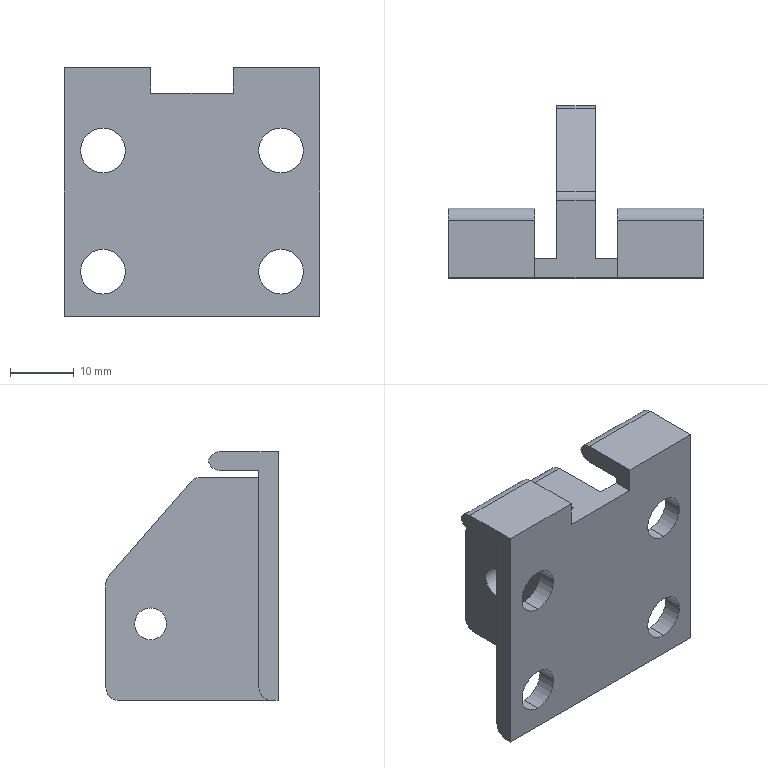Part | SolidWorks | features ICE 4, Extrusion 1, Fillet 1 | 1 solid | 36 faces | box 40 x 27 x 39 mm | volume 8879 mm3 | cylinder 19 | plane 17 | commonest cylinder face diameters 4 x9 7 x8 5 x2
STEP:
#1=CARTESIAN_POINT('',(13.951,3.,-16.5));
#2=VERTEX_POINT('',#1);
#3=CARTESIAN_POINT('',(13.951,3.,-9.5));
#4=VERTEX_POINT('',#3);
#5=CARTESIAN_POINT('',(13.951,3.,-13.));
#6=DIRECTION('',(0.,1.,0.));
#7=DIRECTION('',(0.,0.,-1.));
#8=AXIS2_PLACEMENT_3D('',#5,#6,#7);
#9=CIRCLE('',#8,3.5);
#10=EDGE_CURVE('',#2,#4,#9,.T.);
#11=ORIENTED_EDGE('',*,*,#10,.T.);
#12=CARTESIAN_POINT('',(13.951,0.,-9.5));
#13=VERTEX_POINT('',#12);
#14=CARTESIAN_POINT('',(13.951,27.001,-9.5));
#15=DIRECTION('',(0.,-1.,0.));
#16=VECTOR('',#15,1000.);
#17=LINE('',#14,#16);
#18=EDGE_CURVE('',#4,#13,#17,.T.);
#19=ORIENTED_EDGE('',*,*,#18,.T.);
#20=CARTESIAN_POINT('',(13.951,0.,-16.5));
#21=VERTEX_POINT('',#20);
#22=CARTESIAN_POINT('',(13.951,0.,-13.));
#23=DIRECTION('',(0.,-1.,0.));
#24=DIRECTION('',(0.,0.,1.));
#25=AXIS2_PLACEMENT_3D('',#22,#23,#24);
#26=CIRCLE('',#25,3.5);
#27=EDGE_CURVE('',#13,#21,#26,.T.);
#28=ORIENTED_EDGE('',*,*,#27,.T.);
#29=CARTESIAN_POINT('',(13.951,27.001,-16.5));
#30=DIRECTION('',(0.,-1.,0.));
#31=VECTOR('',#30,1000.);
#32=LINE('',#29,#31);
#33=EDGE_CURVE('',#2,#21,#32,.T.);
#34=ORIENTED_EDGE('',*,*,#33,.F.);
#35=EDGE_LOOP('',(#11,#19,#28,#34));
#36=FACE_OUTER_BOUND('',#35,.T.);
#37=CARTESIAN_POINT('',(13.951,27.001,-13.));
#38=DIRECTION('',(0.,-1.,0.));
#39=DIRECTION('',(0.,0.,-1.));
#40=AXIS2_PLACEMENT_3D('',#37,#38,#39);
#41=CYLINDRICAL_SURFACE('',#40,3.5);
#42=ADVANCED_FACE('',(#36),#41,.F.);
#43=CARTESIAN_POINT('',(13.951,3.,-35.5));
#44=VERTEX_POINT('',#43);
#45=CARTESIAN_POINT('',(13.951,3.,-28.5));
#46=VERTEX_POINT('',#45);
#47=CARTESIAN_POINT('',(13.951,3.,-32.));
#48=DIRECTION('',(0.,1.,0.));
#49=DIRECTION('',(0.,0.,-1.));
#50=AXIS2_PLACEMENT_3D('',#47,#48,#49);
#51=CIRCLE('',#50,3.5);
#52=EDGE_CURVE('',#44,#46,#51,.T.);
#53=ORIENTED_EDGE('',*,*,#52,.T.);
#54=CARTESIAN_POINT('',(13.951,0.,-28.5));
#55=VERTEX_POINT('',#54);
#56=CARTESIAN_POINT('',(13.951,27.001,-28.5));
#57=DIRECTION('',(0.,-1.,0.));
#58=VECTOR('',#57,1000.);
#59=LINE('',#56,#58);
#60=EDGE_CURVE('',#46,#55,#59,.T.);
#61=ORIENTED_EDGE('',*,*,#60,.T.);
#62=CARTESIAN_POINT('',(13.951,0.,-35.5));
#63=VERTEX_POINT('',#62);
#64=CARTESIAN_POINT('',(13.951,0.,-32.));
#65=DIRECTION('',(0.,-1.,0.));
#66=DIRECTION('',(0.,0.,1.));
#67=AXIS2_PLACEMENT_3D('',#64,#65,#66);
#68=CIRCLE('',#67,3.5);
#69=EDGE_CURVE('',#55,#63,#68,.T.);
#70=ORIENTED_EDGE('',*,*,#69,.T.);
#71=CARTESIAN_POINT('',(13.951,27.001,-35.5));
#72=DIRECTION('',(0.,-1.,0.));
#73=VECTOR('',#72,1000.);
#74=LINE('',#71,#73);
#75=EDGE_CURVE('',#44,#63,#74,.T.);
#76=ORIENTED_EDGE('',*,*,#75,.F.);
#77=EDGE_LOOP('',(#53,#61,#70,#76));
#78=FACE_OUTER_BOUND('',#77,.T.);
#79=CARTESIAN_POINT('',(13.951,27.001,-32.));
#80=DIRECTION('',(0.,-1.,0.));
#81=DIRECTION('',(0.,0.,-1.));
#82=AXIS2_PLACEMENT_3D('',#79,#80,#81);
#83=CYLINDRICAL_SURFACE('',#82,3.5);
#84=ADVANCED_FACE('',(#78),#83,.F.);
#85=CARTESIAN_POINT('',(-13.951,3.,-35.5));
#86=VERTEX_POINT('',#85);
#87=CARTESIAN_POINT('',(-13.951,3.,-28.5));
#88=VERTEX_POINT('',#87);
#89=CARTESIAN_POINT('',(-13.951,3.,-32.));
#90=DIRECTION('',(0.,1.,0.));
#91=DIRECTION('',(0.,0.,-1.));
#92=AXIS2_PLACEMENT_3D('',#89,#90,#91);
#93=CIRCLE('',#92,3.5);
#94=EDGE_CURVE('',#86,#88,#93,.T.);
#95=ORIENTED_EDGE('',*,*,#94,.T.);
#96=CARTESIAN_POINT('',(-13.951,0.,-28.5));
#97=VERTEX_POINT('',#96);
#98=CARTESIAN_POINT('',(-13.951,27.001,-28.5));
#99=DIRECTION('',(0.,-1.,0.));
#100=VECTOR('',#99,1000.);
#101=LINE('',#98,#100);
#102=EDGE_CURVE('',#88,#97,#101,.T.);
#103=ORIENTED_EDGE('',*,*,#102,.T.);
#104=CARTESIAN_POINT('',(-13.951,0.,-35.5));
#105=VERTEX_POINT('',#104);
#106=CARTESIAN_POINT('',(-13.951,0.,-32.));
#107=DIRECTION('',(0.,-1.,0.));
#108=DIRECTION('',(0.,0.,-1.));
#109=AXIS2_PLACEMENT_3D('',#106,#107,#108);
#110=CIRCLE('',#109,3.5);
#111=EDGE_CURVE('',#97,#105,#110,.T.);
#112=ORIENTED_EDGE('',*,*,#111,.T.);
#113=CARTESIAN_POINT('',(-13.951,27.001,-35.5));
#114=DIRECTION('',(0.,-1.,0.));
#115=VECTOR('',#114,1000.);
#116=LINE('',#113,#115);
#117=EDGE_CURVE('',#86,#105,#116,.T.);
#118=ORIENTED_EDGE('',*,*,#117,.F.);
#119=EDGE_LOOP('',(#95,#103,#112,#118));
#120=FACE_OUTER_BOUND('',#119,.T.);
#121=CARTESIAN_POINT('',(-13.951,27.001,-32.));
#122=DIRECTION('',(0.,-1.,0.));
#123=DIRECTION('',(0.,0.,-1.));
#124=AXIS2_PLACEMENT_3D('',#121,#122,#123);
#125=CYLINDRICAL_SURFACE('',#124,3.5);
#126=ADVANCED_FACE('',(#120),#125,.F.);
#127=CARTESIAN_POINT('',(-13.951,3.,-16.5));
#128=VERTEX_POINT('',#127);
#129=CARTESIAN_POINT('',(-13.951,3.,-9.5));
#130=VERTEX_POINT('',#129);
#131=CARTESIAN_POINT('',(-13.951,3.,-13.));
#132=DIRECTION('',(0.,1.,0.));
#133=DIRECTION('',(0.,0.,-1.));
#134=AXIS2_PLACEMENT_3D('',#131,#132,#133);
#135=CIRCLE('',#134,3.5);
#136=EDGE_CURVE('',#128,#130,#135,.T.);
#137=ORIENTED_EDGE('',*,*,#136,.T.);
#138=CARTESIAN_POINT('',(-13.951,0.,-9.5));
#139=VERTEX_POINT('',#138);
#140=CARTESIAN_POINT('',(-13.951,27.001,-9.5));
#141=DIRECTION('',(0.,-1.,0.));
#142=VECTOR('',#141,1000.);
#143=LINE('',#140,#142);
#144=EDGE_CURVE('',#130,#139,#143,.T.);
#145=ORIENTED_EDGE('',*,*,#144,.T.);
#146=CARTESIAN_POINT('',(-13.951,0.,-16.5));
#147=VERTEX_POINT('',#146);
#148=CARTESIAN_POINT('',(-13.951,0.,-13.));
#149=DIRECTION('',(0.,-1.,0.));
#150=DIRECTION('',(0.,0.,-1.));
#151=AXIS2_PLACEMENT_3D('',#148,#149,#150);
#152=CIRCLE('',#151,3.5);
#153=EDGE_CURVE('',#139,#147,#152,.T.);
#154=ORIENTED_EDGE('',*,*,#153,.T.);
#155=CARTESIAN_POINT('',(-13.951,27.001,-16.5));
#156=DIRECTION('',(0.,-1.,0.));
#157=VECTOR('',#156,1000.);
#158=LINE('',#155,#157);
#159=EDGE_CURVE('',#128,#147,#158,.T.);
#160=ORIENTED_EDGE('',*,*,#159,.F.);
#161=EDGE_LOOP('',(#137,#145,#154,#160));
#162=FACE_OUTER_BOUND('',#161,.T.);
#163=CARTESIAN_POINT('',(-13.951,27.001,-13.));
#164=DIRECTION('',(0.,-1.,0.));
#165=DIRECTION('',(0.,0.,-1.));
#166=AXIS2_PLACEMENT_3D('',#163,#164,#165);
#167=CYLINDRICAL_SURFACE('',#166,3.5);
#168=ADVANCED_FACE('',(#162),#167,.F.);
#169=CARTESIAN_POINT('',(-3.,20.,-29.5));
#170=VERTEX_POINT('',#169);
#171=CARTESIAN_POINT('',(-3.,20.,-24.5));
#172=VERTEX_POINT('',#171);
#173=CARTESIAN_POINT('',(-3.,20.,-27.));
#174=DIRECTION('',(-1.,0.,0.));
#175=DIRECTION('',(0.,0.,-1.));
#176=AXIS2_PLACEMENT_3D('',#173,#174,#175);
#177=CIRCLE('',#176,2.5);
#178=EDGE_CURVE('',#170,#172,#177,.T.);
#179=ORIENTED_EDGE('',*,*,#178,.T.);
#180=CARTESIAN_POINT('',(3.,20.,-24.5));
#181=VERTEX_POINT('',#180);
#182=CARTESIAN_POINT('',(-20.001,20.,-24.5));
#183=DIRECTION('',(1.,0.,0.));
#184=VECTOR('',#183,1000.);
#185=LINE('',#182,#184);
#186=EDGE_CURVE('',#172,#181,#185,.T.);
#187=ORIENTED_EDGE('',*,*,#186,.T.);
#188=CARTESIAN_POINT('',(3.,20.,-29.5));
#189=VERTEX_POINT('',#188);
#190=CARTESIAN_POINT('',(3.,20.,-27.));
#191=DIRECTION('',(1.,0.,0.));
#192=DIRECTION('',(0.,0.,-1.));
#193=AXIS2_PLACEMENT_3D('',#190,#191,#192);
#194=CIRCLE('',#193,2.5);
#195=EDGE_CURVE('',#181,#189,#194,.T.);
#196=ORIENTED_EDGE('',*,*,#195,.T.);
#197=CARTESIAN_POINT('',(-20.001,20.,-29.5));
#198=DIRECTION('',(1.,0.,0.));
#199=VECTOR('',#198,1000.);
#200=LINE('',#197,#199);
#201=EDGE_CURVE('',#170,#189,#200,.T.);
#202=ORIENTED_EDGE('',*,*,#201,.F.);
#203=EDGE_LOOP('',(#179,#187,#196,#202));
#204=FACE_OUTER_BOUND('',#203,.T.);
#205=CARTESIAN_POINT('',(-20.001,20.,-27.));
#206=DIRECTION('',(1.,0.,0.));
#207=DIRECTION('',(0.,0.,-1.));
#208=AXIS2_PLACEMENT_3D('',#205,#206,#207);
#209=CYLINDRICAL_SURFACE('',#208,2.5);
#210=ADVANCED_FACE('',(#204),#209,.F.);
#211=ORIENTED_EDGE('',*,*,#94,.F.);
#212=CARTESIAN_POINT('',(-13.951,3.,-32.));
#213=DIRECTION('',(0.,1.,0.));
#214=DIRECTION('',(0.,0.,-1.));
#215=AXIS2_PLACEMENT_3D('',#212,#213,#214);
#216=CIRCLE('',#215,3.5);
#217=EDGE_CURVE('',#88,#86,#216,.T.);
#218=ORIENTED_EDGE('',*,*,#217,.F.);
#219=EDGE_LOOP('',(#211,#218));
#220=FACE_BOUND('',#219,.T.);
#221=ORIENTED_EDGE('',*,*,#136,.F.);
#222=CARTESIAN_POINT('',(-13.951,3.,-13.));
#223=DIRECTION('',(0.,1.,0.));
#224=DIRECTION('',(0.,0.,-1.));
#225=AXIS2_PLACEMENT_3D('',#222,#223,#224);
#226=CIRCLE('',#225,3.5);
#227=EDGE_CURVE('',#130,#128,#226,.T.);
#228=ORIENTED_EDGE('',*,*,#227,.F.);
#229=EDGE_LOOP('',(#221,#228));
#230=FACE_BOUND('',#229,.T.);
#231=CARTESIAN_POINT('',(-3.,3.,-4.));
#232=VERTEX_POINT('',#231);
#233=CARTESIAN_POINT('',(-3.,3.,-37.));
#234=VERTEX_POINT('',#233);
#235=CARTESIAN_POINT('',(-3.,3.,-4.));
#236=DIRECTION('',(0.,0.,-1.));
#237=VECTOR('',#236,1000.);
#238=LINE('',#235,#237);
#239=EDGE_CURVE('',#232,#234,#238,.T.);
#240=ORIENTED_EDGE('',*,*,#239,.T.);
#241=CARTESIAN_POINT('',(-20.,3.,-37.));
#242=VERTEX_POINT('',#241);
#243=CARTESIAN_POINT('',(20.,3.,-37.));
#244=DIRECTION('',(-1.,0.,0.));
#245=VECTOR('',#244,1000.);
#246=LINE('',#243,#245);
#247=EDGE_CURVE('',#234,#242,#246,.T.);
#248=ORIENTED_EDGE('',*,*,#247,.T.);
#249=CARTESIAN_POINT('',(-20.,3.,-3.));
#250=VERTEX_POINT('',#249);
#251=CARTESIAN_POINT('',(-20.,3.,0.));
#252=DIRECTION('',(0.,0.,1.));
#253=VECTOR('',#252,1000.);
#254=LINE('',#251,#253);
#255=EDGE_CURVE('',#242,#250,#254,.T.);
#256=ORIENTED_EDGE('',*,*,#255,.T.);
#257=CARTESIAN_POINT('',(-6.5,3.,-3.));
#258=VERTEX_POINT('',#257);
#259=CARTESIAN_POINT('',(20.,3.,-3.));
#260=DIRECTION('',(-1.,0.,0.));
#261=VECTOR('',#260,1000.);
#262=LINE('',#259,#261);
#263=EDGE_CURVE('',#258,#250,#262,.T.);
#264=ORIENTED_EDGE('',*,*,#263,.F.);
#265=CARTESIAN_POINT('',(-6.5,3.,-4.));
#266=VERTEX_POINT('',#265);
#267=CARTESIAN_POINT('',(-6.5,3.,0.));
#268=DIRECTION('',(0.,0.,1.));
#269=VECTOR('',#268,1000.);
#270=LINE('',#267,#269);
#271=EDGE_CURVE('',#266,#258,#270,.T.);
#272=ORIENTED_EDGE('',*,*,#271,.F.);
#273=CARTESIAN_POINT('',(20.,3.,-4.));
#274=DIRECTION('',(1.,0.,0.));
#275=VECTOR('',#274,1000.);
#276=LINE('',#273,#275);
#277=EDGE_CURVE('',#266,#232,#276,.T.);
#278=ORIENTED_EDGE('',*,*,#277,.T.);
#279=EDGE_LOOP('',(#240,#248,#256,#264,#272,#278));
#280=FACE_OUTER_BOUND('',#279,.T.);
#281=CARTESIAN_POINT('',(20.,3.,0.));
#282=DIRECTION('',(0.,-1.,0.));
#283=DIRECTION('',(0.,0.,-1.));
#284=AXIS2_PLACEMENT_3D('',#281,#282,#283);
#285=PLANE('',#284);
#286=ADVANCED_FACE('',(#220,#230,#280),#285,.F.);
#287=CARTESIAN_POINT('',(-20.,9.,-3.));
#288=VERTEX_POINT('',#287);
#289=CARTESIAN_POINT('',(-20.,0.,-3.));
#290=DIRECTION('',(0.,-1.,0.));
#291=VECTOR('',#290,1000.);
#292=LINE('',#289,#291);
#293=EDGE_CURVE('',#288,#250,#292,.T.);
#294=ORIENTED_EDGE('',*,*,#293,.F.);
#295=CARTESIAN_POINT('',(-6.5,9.,-3.));
#296=VERTEX_POINT('',#295);
#297=CARTESIAN_POINT('',(20.,9.,-3.));
#298=DIRECTION('',(1.,0.,0.));
#299=VECTOR('',#298,1000.);
#300=LINE('',#297,#299);
#301=EDGE_CURVE('',#288,#296,#300,.T.);
#302=ORIENTED_EDGE('',*,*,#301,.T.);
#303=CARTESIAN_POINT('',(-6.5,0.,-3.));
#304=DIRECTION('',(0.,-1.,0.));
#305=VECTOR('',#304,1000.);
#306=LINE('',#303,#305);
#307=EDGE_CURVE('',#296,#258,#306,.T.);
#308=ORIENTED_EDGE('',*,*,#307,.T.);
#309=ORIENTED_EDGE('',*,*,#263,.T.);
#310=EDGE_LOOP('',(#294,#302,#308,#309));
#311=FACE_OUTER_BOUND('',#310,.T.);
#312=CARTESIAN_POINT('',(20.,0.,-3.));
#313=DIRECTION('',(0.,0.,-1.));
#314=DIRECTION('',(-1.,0.,0.));
#315=AXIS2_PLACEMENT_3D('',#312,#313,#314);
#316=PLANE('',#315);
#317=ADVANCED_FACE('',(#311),#316,.T.);
#318=CARTESIAN_POINT('',(-6.5,9.,0.));
#319=VERTEX_POINT('',#318);
#320=CARTESIAN_POINT('',(-6.5,0.,0.));
#321=VERTEX_POINT('',#320);
#322=CARTESIAN_POINT('',(-6.5,11.,0.));
#323=DIRECTION('',(0.,-1.,0.));
#324=VECTOR('',#323,1000.);
#325=LINE('',#322,#324);
#326=EDGE_CURVE('',#319,#321,#325,.T.);
#327=ORIENTED_EDGE('',*,*,#326,.F.);
#328=CARTESIAN_POINT('',(-20.,9.,0.));
#329=VERTEX_POINT('',#328);
#330=CARTESIAN_POINT('',(20.,9.,0.));
#331=DIRECTION('',(-1.,0.,0.));
#332=VECTOR('',#331,1000.);
#333=LINE('',#330,#332);
#334=EDGE_CURVE('',#319,#329,#333,.T.);
#335=ORIENTED_EDGE('',*,*,#334,.T.);
#336=CARTESIAN_POINT('',(-20.,0.,0.));
#337=VERTEX_POINT('',#336);
#338=CARTESIAN_POINT('',(-20.,0.,0.));
#339=DIRECTION('',(0.,1.,0.));
#340=VECTOR('',#339,1000.);
#341=LINE('',#338,#340);
#342=EDGE_CURVE('',#337,#329,#341,.T.);
#343=ORIENTED_EDGE('',*,*,#342,.F.);
#344=CARTESIAN_POINT('',(20.,0.,0.));
#345=DIRECTION('',(-1.,0.,0.));
#346=VECTOR('',#345,1000.);
#347=LINE('',#344,#346);
#348=EDGE_CURVE('',#321,#337,#347,.T.);
#349=ORIENTED_EDGE('',*,*,#348,.F.);
#350=EDGE_LOOP('',(#327,#335,#343,#349));
#351=FACE_OUTER_BOUND('',#350,.T.);
#352=CARTESIAN_POINT('',(20.,0.,0.));
#353=DIRECTION('',(0.,0.,1.));
#354=DIRECTION('',(1.,0.,0.));
#355=AXIS2_PLACEMENT_3D('',#352,#353,#354);
#356=PLANE('',#355);
#357=ADVANCED_FACE('',(#351),#356,.T.);
#358=CARTESIAN_POINT('',(13.951,0.,-13.));
#359=DIRECTION('',(0.,-1.,0.));
#360=DIRECTION('',(0.,0.,1.));
#361=AXIS2_PLACEMENT_3D('',#358,#359,#360);
#362=CIRCLE('',#361,3.5);
#363=EDGE_CURVE('',#21,#13,#362,.T.);
#364=ORIENTED_EDGE('',*,*,#363,.F.);
#365=ORIENTED_EDGE('',*,*,#27,.F.);
#366=EDGE_LOOP('',(#364,#365));
#367=FACE_BOUND('',#366,.T.);
#368=CARTESIAN_POINT('',(13.951,0.,-32.));
#369=DIRECTION('',(0.,-1.,0.));
#370=DIRECTION('',(0.,0.,1.));
#371=AXIS2_PLACEMENT_3D('',#368,#369,#370);
#372=CIRCLE('',#371,3.5);
#373=EDGE_CURVE('',#63,#55,#372,.T.);
#374=ORIENTED_EDGE('',*,*,#373,.F.);
#375=ORIENTED_EDGE('',*,*,#69,.F.);
#376=EDGE_LOOP('',(#374,#375));
#377=FACE_BOUND('',#376,.T.);
#378=CARTESIAN_POINT('',(-13.951,0.,-32.));
#379=DIRECTION('',(0.,-1.,0.));
#380=DIRECTION('',(0.,0.,-1.));
#381=AXIS2_PLACEMENT_3D('',#378,#379,#380);
#382=CIRCLE('',#381,3.5);
#383=EDGE_CURVE('',#105,#97,#382,.T.);
#384=ORIENTED_EDGE('',*,*,#383,.F.);
#385=ORIENTED_EDGE('',*,*,#111,.F.);
#386=EDGE_LOOP('',(#384,#385));
#387=FACE_BOUND('',#386,.T.);
#388=CARTESIAN_POINT('',(-13.951,0.,-13.));
#389=DIRECTION('',(0.,-1.,0.));
#390=DIRECTION('',(0.,0.,-1.));
#391=AXIS2_PLACEMENT_3D('',#388,#389,#390);
#392=CIRCLE('',#391,3.5);
#393=EDGE_CURVE('',#147,#139,#392,.T.);
#394=ORIENTED_EDGE('',*,*,#393,.F.);
#395=ORIENTED_EDGE('',*,*,#153,.F.);
#396=EDGE_LOOP('',(#394,#395));
#397=FACE_BOUND('',#396,.T.);
#398=CARTESIAN_POINT('',(-6.5,0.,-4.));
#399=VERTEX_POINT('',#398);
#400=CARTESIAN_POINT('',(-6.5,0.,0.));
#401=DIRECTION('',(0.,0.,-1.));
#402=VECTOR('',#401,1000.);
#403=LINE('',#400,#402);
#404=EDGE_CURVE('',#321,#399,#403,.T.);
#405=ORIENTED_EDGE('',*,*,#404,.F.);
#406=ORIENTED_EDGE('',*,*,#348,.T.);
#407=CARTESIAN_POINT('',(-20.,0.,-39.));
#408=VERTEX_POINT('',#407);
#409=CARTESIAN_POINT('',(-20.,0.,0.));
#410=DIRECTION('',(0.,0.,-1.));
#411=VECTOR('',#410,1000.);
#412=LINE('',#409,#411);
#413=EDGE_CURVE('',#337,#408,#412,.T.);
#414=ORIENTED_EDGE('',*,*,#413,.T.);
#415=CARTESIAN_POINT('',(20.,0.,-39.));
#416=VERTEX_POINT('',#415);
#417=CARTESIAN_POINT('',(20.,0.,-39.));
#418=DIRECTION('',(-1.,0.,0.));
#419=VECTOR('',#418,1000.);
#420=LINE('',#417,#419);
#421=EDGE_CURVE('',#416,#408,#420,.T.);
#422=ORIENTED_EDGE('',*,*,#421,.F.);
#423=CARTESIAN_POINT('',(20.,0.,0.));
#424=VERTEX_POINT('',#423);
#425=CARTESIAN_POINT('',(20.,0.,0.));
#426=DIRECTION('',(0.,0.,-1.));
#427=VECTOR('',#426,1000.);
#428=LINE('',#425,#427);
#429=EDGE_CURVE('',#424,#416,#428,.T.);
#430=ORIENTED_EDGE('',*,*,#429,.F.);
#431=CARTESIAN_POINT('',(6.5,0.,0.));
#432=VERTEX_POINT('',#431);
#433=CARTESIAN_POINT('',(20.,0.,0.));
#434=DIRECTION('',(-1.,0.,0.));
#435=VECTOR('',#434,1000.);
#436=LINE('',#433,#435);
#437=EDGE_CURVE('',#424,#432,#436,.T.);
#438=ORIENTED_EDGE('',*,*,#437,.T.);
#439=CARTESIAN_POINT('',(6.5,0.,-4.));
#440=VERTEX_POINT('',#439);
#441=CARTESIAN_POINT('',(6.5,0.,0.));
#442=DIRECTION('',(0.,0.,-1.));
#443=VECTOR('',#442,1000.);
#444=LINE('',#441,#443);
#445=EDGE_CURVE('',#432,#440,#444,.T.);
#446=ORIENTED_EDGE('',*,*,#445,.T.);
#447=CARTESIAN_POINT('',(-6.5,0.,-4.));
#448=DIRECTION('',(1.,0.,0.));
#449=VECTOR('',#448,1000.);
#450=LINE('',#447,#449);
#451=EDGE_CURVE('',#399,#440,#450,.T.);
#452=ORIENTED_EDGE('',*,*,#451,.F.);
#453=EDGE_LOOP('',(#405,#406,#414,#422,#430,#438,#446,#452));
#454=FACE_OUTER_BOUND('',#453,.T.);
#455=CARTESIAN_POINT('',(20.,0.,0.));
#456=DIRECTION('',(0.,1.,0.));
#457=DIRECTION('',(0.,0.,1.));
#458=AXIS2_PLACEMENT_3D('',#455,#456,#457);
#459=PLANE('',#458);
#460=ADVANCED_FACE('',(#367,#377,#387,#397,#454),#459,.F.);
#461=ORIENTED_EDGE('',*,*,#10,.F.);
#462=CARTESIAN_POINT('',(13.951,3.,-13.));
#463=DIRECTION('',(0.,1.,0.));
#464=DIRECTION('',(0.,0.,-1.));
#465=AXIS2_PLACEMENT_3D('',#462,#463,#464);
#466=CIRCLE('',#465,3.5);
#467=EDGE_CURVE('',#4,#2,#466,.T.);
#468=ORIENTED_EDGE('',*,*,#467,.F.);
#469=EDGE_LOOP('',(#461,#468));
#470=FACE_BOUND('',#469,.T.);
#471=ORIENTED_EDGE('',*,*,#52,.F.);
#472=CARTESIAN_POINT('',(13.951,3.,-32.));
#473=DIRECTION('',(0.,1.,0.));
#474=DIRECTION('',(0.,0.,-1.));
#475=AXIS2_PLACEMENT_3D('',#472,#473,#474);
#476=CIRCLE('',#475,3.5);
#477=EDGE_CURVE('',#46,#44,#476,.T.);
#478=ORIENTED_EDGE('',*,*,#477,.F.);
#479=EDGE_LOOP('',(#471,#478));
#480=FACE_BOUND('',#479,.T.);
#481=CARTESIAN_POINT('',(20.,3.,-37.));
#482=VERTEX_POINT('',#481);
#483=CARTESIAN_POINT('',(20.,3.,-3.));
#484=VERTEX_POINT('',#483);
#485=CARTESIAN_POINT('',(20.,3.,0.));
#486=DIRECTION('',(0.,0.,1.));
#487=VECTOR('',#486,1000.);
#488=LINE('',#485,#487);
#489=EDGE_CURVE('',#482,#484,#488,.T.);
#490=ORIENTED_EDGE('',*,*,#489,.F.);
#491=CARTESIAN_POINT('',(3.,3.,-37.));
#492=VERTEX_POINT('',#491);
#493=CARTESIAN_POINT('',(20.,3.,-37.));
#494=DIRECTION('',(-1.,0.,0.));
#495=VECTOR('',#494,1000.);
#496=LINE('',#493,#495);
#497=EDGE_CURVE('',#482,#492,#496,.T.);
#498=ORIENTED_EDGE('',*,*,#497,.T.);
#499=CARTESIAN_POINT('',(3.,3.,-4.));
#500=VERTEX_POINT('',#499);
#501=CARTESIAN_POINT('',(3.,3.,-4.));
#502=DIRECTION('',(0.,0.,-1.));
#503=VECTOR('',#502,1000.);
#504=LINE('',#501,#503);
#505=EDGE_CURVE('',#500,#492,#504,.T.);
#506=ORIENTED_EDGE('',*,*,#505,.F.);
#507=CARTESIAN_POINT('',(6.5,3.,-4.));
#508=VERTEX_POINT('',#507);
#509=CARTESIAN_POINT('',(20.,3.,-4.));
#510=DIRECTION('',(1.,0.,0.));
#511=VECTOR('',#510,1000.);
#512=LINE('',#509,#511);
#513=EDGE_CURVE('',#500,#508,#512,.T.);
#514=ORIENTED_EDGE('',*,*,#513,.T.);
#515=CARTESIAN_POINT('',(6.5,3.,-3.));
#516=VERTEX_POINT('',#515);
#517=CARTESIAN_POINT('',(6.5,3.,0.));
#518=DIRECTION('',(0.,0.,1.));
#519=VECTOR('',#518,1000.);
#520=LINE('',#517,#519);
#521=EDGE_CURVE('',#508,#516,#520,.T.);
#522=ORIENTED_EDGE('',*,*,#521,.T.);
#523=CARTESIAN_POINT('',(20.,3.,-3.));
#524=DIRECTION('',(-1.,0.,0.));
#525=VECTOR('',#524,1000.);
#526=LINE('',#523,#525);
#527=EDGE_CURVE('',#484,#516,#526,.T.);
#528=ORIENTED_EDGE('',*,*,#527,.F.);
#529=EDGE_LOOP('',(#490,#498,#506,#514,#522,#528));
#530=FACE_OUTER_BOUND('',#529,.T.);
#531=CARTESIAN_POINT('',(20.,3.,0.));
#532=DIRECTION('',(0.,-1.,0.));
#533=DIRECTION('',(0.,0.,-1.));
#534=AXIS2_PLACEMENT_3D('',#531,#532,#533);
#535=PLANE('',#534);
#536=ADVANCED_FACE('',(#470,#480,#530),#535,.F.);
#537=CARTESIAN_POINT('',(6.5,9.,-3.));
#538=VERTEX_POINT('',#537);
#539=CARTESIAN_POINT('',(6.5,0.,-3.));
#540=DIRECTION('',(0.,-1.,0.));
#541=VECTOR('',#540,1000.);
#542=LINE('',#539,#541);
#543=EDGE_CURVE('',#538,#516,#542,.T.);
#544=ORIENTED_EDGE('',*,*,#543,.F.);
#545=CARTESIAN_POINT('',(20.,9.,-3.));
#546=VERTEX_POINT('',#545);
#547=CARTESIAN_POINT('',(20.,9.,-3.));
#548=DIRECTION('',(1.,0.,0.));
#549=VECTOR('',#548,1000.);
#550=LINE('',#547,#549);
#551=EDGE_CURVE('',#538,#546,#550,.T.);
#552=ORIENTED_EDGE('',*,*,#551,.T.);
#553=CARTESIAN_POINT('',(20.,0.,-3.));
#554=DIRECTION('',(0.,-1.,0.));
#555=VECTOR('',#554,1000.);
#556=LINE('',#553,#555);
#557=EDGE_CURVE('',#546,#484,#556,.T.);
#558=ORIENTED_EDGE('',*,*,#557,.T.);
#559=ORIENTED_EDGE('',*,*,#527,.T.);
#560=EDGE_LOOP('',(#544,#552,#558,#559));
#561=FACE_OUTER_BOUND('',#560,.T.);
#562=CARTESIAN_POINT('',(20.,0.,-3.));
#563=DIRECTION('',(0.,0.,-1.));
#564=DIRECTION('',(-1.,0.,0.));
#565=AXIS2_PLACEMENT_3D('',#562,#563,#564);
#566=PLANE('',#565);
#567=ADVANCED_FACE('',(#561),#566,.T.);
#568=CARTESIAN_POINT('',(20.,9.,0.));
#569=VERTEX_POINT('',#568);
#570=CARTESIAN_POINT('',(20.,0.,0.));
#571=DIRECTION('',(0.,1.,0.));
#572=VECTOR('',#571,1000.);
#573=LINE('',#570,#572);
#574=EDGE_CURVE('',#424,#569,#573,.T.);
#575=ORIENTED_EDGE('',*,*,#574,.T.);
#576=CARTESIAN_POINT('',(6.5,9.,0.));
#577=VERTEX_POINT('',#576);
#578=CARTESIAN_POINT('',(20.,9.,0.));
#579=DIRECTION('',(-1.,0.,0.));
#580=VECTOR('',#579,1000.);
#581=LINE('',#578,#580);
#582=EDGE_CURVE('',#569,#577,#581,.T.);
#583=ORIENTED_EDGE('',*,*,#582,.T.);
#584=CARTESIAN_POINT('',(6.5,11.,0.));
#585=DIRECTION('',(0.,-1.,0.));
#586=VECTOR('',#585,1000.);
#587=LINE('',#584,#586);
#588=EDGE_CURVE('',#577,#432,#587,.T.);
#589=ORIENTED_EDGE('',*,*,#588,.T.);
#590=ORIENTED_EDGE('',*,*,#437,.F.);
#591=EDGE_LOOP('',(#575,#583,#589,#590));
#592=FACE_OUTER_BOUND('',#591,.T.);
#593=CARTESIAN_POINT('',(20.,0.,0.));
#594=DIRECTION('',(0.,0.,1.));
#595=DIRECTION('',(1.,0.,0.));
#596=AXIS2_PLACEMENT_3D('',#593,#594,#595);
#597=PLANE('',#596);
#598=ADVANCED_FACE('',(#592),#597,.T.);
#599=CARTESIAN_POINT('',(-20.,1.,-39.));
#600=VERTEX_POINT('',#599);
#601=CARTESIAN_POINT('',(-20.,0.,-39.));
#602=DIRECTION('',(0.,1.,0.));
#603=VECTOR('',#602,1000.);
#604=LINE('',#601,#603);
#605=EDGE_CURVE('',#408,#600,#604,.T.);
#606=ORIENTED_EDGE('',*,*,#605,.T.);
#607=CARTESIAN_POINT('',(-3.,1.,-39.));
#608=VERTEX_POINT('',#607);
#609=CARTESIAN_POINT('',(20.,1.,-39.));
#610=DIRECTION('',(1.,0.,0.));
#611=VECTOR('',#610,1000.);
#612=LINE('',#609,#611);
#613=EDGE_CURVE('',#600,#608,#612,.T.);
#614=ORIENTED_EDGE('',*,*,#613,.T.);
#615=CARTESIAN_POINT('',(-3.,25.,-39.));
#616=VERTEX_POINT('',#615);
#617=CARTESIAN_POINT('',(-3.,3.,-39.));
#618=DIRECTION('',(0.,1.,0.));
#619=VECTOR('',#618,1000.);
#620=LINE('',#617,#619);
#621=EDGE_CURVE('',#608,#616,#620,.T.);
#622=ORIENTED_EDGE('',*,*,#621,.T.);
#623=CARTESIAN_POINT('',(3.,25.,-39.));
#624=VERTEX_POINT('',#623);
#625=CARTESIAN_POINT('',(20.,25.,-39.));
#626=DIRECTION('',(1.,0.,0.));
#627=VECTOR('',#626,1000.);
#628=LINE('',#625,#627);
#629=EDGE_CURVE('',#616,#624,#628,.T.);
#630=ORIENTED_EDGE('',*,*,#629,.T.);
#631=CARTESIAN_POINT('',(3.,1.,-39.));
#632=VERTEX_POINT('',#631);
#633=CARTESIAN_POINT('',(3.,3.,-39.));
#634=DIRECTION('',(0.,1.,0.));
#635=VECTOR('',#634,1000.);
#636=LINE('',#633,#635);
#637=EDGE_CURVE('',#632,#624,#636,.T.);
#638=ORIENTED_EDGE('',*,*,#637,.F.);
#639=CARTESIAN_POINT('',(20.,1.,-39.));
#640=VERTEX_POINT('',#639);
#641=CARTESIAN_POINT('',(20.,1.,-39.));
#642=DIRECTION('',(1.,0.,0.));
#643=VECTOR('',#642,1000.);
#644=LINE('',#641,#643);
#645=EDGE_CURVE('',#632,#640,#644,.T.);
#646=ORIENTED_EDGE('',*,*,#645,.T.);
#647=CARTESIAN_POINT('',(20.,0.,-39.));
#648=DIRECTION('',(0.,1.,0.));
#649=VECTOR('',#648,1000.);
#650=LINE('',#647,#649);
#651=EDGE_CURVE('',#416,#640,#650,.T.);
#652=ORIENTED_EDGE('',*,*,#651,.F.);
#653=ORIENTED_EDGE('',*,*,#421,.T.);
#654=EDGE_LOOP('',(#606,#614,#622,#630,#638,#646,#652,#653));
#655=FACE_OUTER_BOUND('',#654,.T.);
#656=CARTESIAN_POINT('',(20.,0.,-39.));
#657=DIRECTION('',(0.,0.,1.));
#658=DIRECTION('',(1.,0.,0.));
#659=AXIS2_PLACEMENT_3D('',#656,#657,#658);
#660=PLANE('',#659);
#661=ADVANCED_FACE('',(#655),#660,.F.);
#662=ORIENTED_EDGE('',*,*,#651,.T.);
#663=CARTESIAN_POINT('',(20.,1.,-37.));
#664=DIRECTION('',(1.,0.,0.));
#665=DIRECTION('',(0.,0.,-1.));
#666=AXIS2_PLACEMENT_3D('',#663,#664,#665);
#667=CIRCLE('',#666,2.);
#668=EDGE_CURVE('',#640,#482,#667,.T.);
#669=ORIENTED_EDGE('',*,*,#668,.T.);
#670=ORIENTED_EDGE('',*,*,#489,.T.);
#671=ORIENTED_EDGE('',*,*,#557,.F.);
#672=CARTESIAN_POINT('',(20.,10.936,-1.5));
#673=VERTEX_POINT('',#672);
#674=CARTESIAN_POINT('',(20.,9.,-1.));
#675=DIRECTION('',(1.,0.,0.));
#676=DIRECTION('',(0.,0.,-1.));
#677=AXIS2_PLACEMENT_3D('',#674,#675,#676);
#678=CIRCLE('',#677,2.);
#679=EDGE_CURVE('',#546,#673,#678,.T.);
#680=ORIENTED_EDGE('',*,*,#679,.T.);
#681=CARTESIAN_POINT('',(20.,9.,-2.));
#682=DIRECTION('',(1.,0.,0.));
#683=DIRECTION('',(0.,0.,-1.));
#684=AXIS2_PLACEMENT_3D('',#681,#682,#683);
#685=CIRCLE('',#684,2.);
#686=EDGE_CURVE('',#673,#569,#685,.T.);
#687=ORIENTED_EDGE('',*,*,#686,.T.);
#688=ORIENTED_EDGE('',*,*,#574,.F.);
#689=ORIENTED_EDGE('',*,*,#429,.T.);
#690=EDGE_LOOP('',(#662,#669,#670,#671,#680,#687,#688,#689));
#691=FACE_OUTER_BOUND('',#690,.T.);
#692=CARTESIAN_POINT('',(20.,0.,0.));
#693=DIRECTION('',(1.,0.,0.));
#694=DIRECTION('',(0.,0.,-1.));
#695=AXIS2_PLACEMENT_3D('',#692,#693,#694);
#696=PLANE('',#695);
#697=ADVANCED_FACE('',(#691),#696,.T.);
#698=ORIENTED_EDGE('',*,*,#255,.F.);
#699=CARTESIAN_POINT('',(-20.,1.,-37.));
#700=DIRECTION('',(-1.,0.,0.));
#701=DIRECTION('',(0.,0.,-1.));
#702=AXIS2_PLACEMENT_3D('',#699,#700,#701);
#703=CIRCLE('',#702,2.);
#704=EDGE_CURVE('',#242,#600,#703,.T.);
#705=ORIENTED_EDGE('',*,*,#704,.T.);
#706=ORIENTED_EDGE('',*,*,#605,.F.);
#707=ORIENTED_EDGE('',*,*,#413,.F.);
#708=ORIENTED_EDGE('',*,*,#342,.T.);
#709=CARTESIAN_POINT('',(-20.,10.936,-1.5));
#710=VERTEX_POINT('',#709);
#711=CARTESIAN_POINT('',(-20.,9.,-2.));
#712=DIRECTION('',(-1.,0.,0.));
#713=DIRECTION('',(0.,0.,-1.));
#714=AXIS2_PLACEMENT_3D('',#711,#712,#713);
#715=CIRCLE('',#714,2.);
#716=EDGE_CURVE('',#329,#710,#715,.T.);
#717=ORIENTED_EDGE('',*,*,#716,.T.);
#718=CARTESIAN_POINT('',(-20.,9.,-1.));
#719=DIRECTION('',(-1.,0.,0.));
#720=DIRECTION('',(0.,0.,-1.));
#721=AXIS2_PLACEMENT_3D('',#718,#719,#720);
#722=CIRCLE('',#721,2.);
#723=EDGE_CURVE('',#710,#288,#722,.T.);
#724=ORIENTED_EDGE('',*,*,#723,.T.);
#725=ORIENTED_EDGE('',*,*,#293,.T.);
#726=EDGE_LOOP('',(#698,#705,#706,#707,#708,#717,#724,#725));
#727=FACE_OUTER_BOUND('',#726,.T.);
#728=CARTESIAN_POINT('',(-20.,0.,0.));
#729=DIRECTION('',(1.,0.,0.));
#730=DIRECTION('',(0.,0.,-1.));
#731=AXIS2_PLACEMENT_3D('',#728,#729,#730);
#732=PLANE('',#731);
#733=ADVANCED_FACE('',(#727),#732,.F.);
#734=CARTESIAN_POINT('',(3.,12.092,-4.));
#735=VERTEX_POINT('',#734);
#736=CARTESIAN_POINT('',(3.,13.,-4.));
#737=DIRECTION('',(0.,-1.,0.));
#738=VECTOR('',#737,1000.);
#739=LINE('',#736,#738);
#740=EDGE_CURVE('',#735,#500,#739,.T.);
#741=ORIENTED_EDGE('',*,*,#740,.F.);
#742=CARTESIAN_POINT('',(-3.,12.092,-4.));
#743=VERTEX_POINT('',#742);
#744=CARTESIAN_POINT('',(-6.5,12.092,-4.));
#745=DIRECTION('',(-1.,0.,0.));
#746=VECTOR('',#745,1000.);
#747=LINE('',#744,#746);
#748=EDGE_CURVE('',#735,#743,#747,.T.);
#749=ORIENTED_EDGE('',*,*,#748,.T.);
#750=CARTESIAN_POINT('',(-3.,13.,-4.));
#751=DIRECTION('',(0.,-1.,0.));
#752=VECTOR('',#751,1000.);
#753=LINE('',#750,#752);
#754=EDGE_CURVE('',#743,#232,#753,.T.);
#755=ORIENTED_EDGE('',*,*,#754,.T.);
#756=ORIENTED_EDGE('',*,*,#277,.F.);
#757=CARTESIAN_POINT('',(-6.5,11.,-4.));
#758=DIRECTION('',(0.,1.,0.));
#759=VECTOR('',#758,1000.);
#760=LINE('',#757,#759);
#761=EDGE_CURVE('',#399,#266,#760,.T.);
#762=ORIENTED_EDGE('',*,*,#761,.F.);
#763=ORIENTED_EDGE('',*,*,#451,.T.);
#764=CARTESIAN_POINT('',(6.5,11.,-4.));
#765=DIRECTION('',(0.,1.,0.));
#766=VECTOR('',#765,1000.);
#767=LINE('',#764,#766);
#768=EDGE_CURVE('',#440,#508,#767,.T.);
#769=ORIENTED_EDGE('',*,*,#768,.T.);
#770=ORIENTED_EDGE('',*,*,#513,.F.);
#771=EDGE_LOOP('',(#741,#749,#755,#756,#762,#763,#769,#770));
#772=FACE_OUTER_BOUND('',#771,.T.);
#773=CARTESIAN_POINT('',(-6.5,11.,-4.));
#774=DIRECTION('',(0.,0.,-1.));
#775=DIRECTION('',(0.,1.,0.));
#776=AXIS2_PLACEMENT_3D('',#773,#774,#775);
#777=PLANE('',#776);
#778=ADVANCED_FACE('',(#772),#777,.F.);
#779=ORIENTED_EDGE('',*,*,#307,.F.);
#780=CARTESIAN_POINT('',(-6.5,10.936,-1.5));
#781=VERTEX_POINT('',#780);
#782=CARTESIAN_POINT('',(-6.5,9.,-1.));
#783=DIRECTION('',(1.,0.,0.));
#784=DIRECTION('',(0.,0.,-1.));
#785=AXIS2_PLACEMENT_3D('',#782,#783,#784);
#786=CIRCLE('',#785,2.);
#787=EDGE_CURVE('',#296,#781,#786,.T.);
#788=ORIENTED_EDGE('',*,*,#787,.T.);
#789=CARTESIAN_POINT('',(-6.5,9.,-2.));
#790=DIRECTION('',(1.,0.,0.));
#791=DIRECTION('',(0.,0.,-1.));
#792=AXIS2_PLACEMENT_3D('',#789,#790,#791);
#793=CIRCLE('',#792,2.);
#794=EDGE_CURVE('',#781,#319,#793,.T.);
#795=ORIENTED_EDGE('',*,*,#794,.T.);
#796=ORIENTED_EDGE('',*,*,#326,.T.);
#797=ORIENTED_EDGE('',*,*,#404,.T.);
#798=ORIENTED_EDGE('',*,*,#761,.T.);
#799=ORIENTED_EDGE('',*,*,#271,.T.);
#800=EDGE_LOOP('',(#779,#788,#795,#796,#797,#798,#799));
#801=FACE_OUTER_BOUND('',#800,.T.);
#802=CARTESIAN_POINT('',(-6.5,0.,0.));
#803=DIRECTION('',(1.,0.,0.));
#804=DIRECTION('',(0.,0.,-1.));
#805=AXIS2_PLACEMENT_3D('',#802,#803,#804);
#806=PLANE('',#805);
#807=ADVANCED_FACE('',(#801),#806,.T.);
#808=CARTESIAN_POINT('',(6.5,10.936,-1.5));
#809=VERTEX_POINT('',#808);
#810=CARTESIAN_POINT('',(6.5,9.,-2.));
#811=DIRECTION('',(-1.,0.,0.));
#812=DIRECTION('',(0.,0.,-1.));
#813=AXIS2_PLACEMENT_3D('',#810,#811,#812);
#814=CIRCLE('',#813,2.);
#815=EDGE_CURVE('',#577,#809,#814,.T.);
#816=ORIENTED_EDGE('',*,*,#815,.T.);
#817=CARTESIAN_POINT('',(6.5,9.,-1.));
#818=DIRECTION('',(-1.,0.,0.));
#819=DIRECTION('',(0.,0.,-1.));
#820=AXIS2_PLACEMENT_3D('',#817,#818,#819);
#821=CIRCLE('',#820,2.);
#822=EDGE_CURVE('',#809,#538,#821,.T.);
#823=ORIENTED_EDGE('',*,*,#822,.T.);
#824=ORIENTED_EDGE('',*,*,#543,.T.);
#825=ORIENTED_EDGE('',*,*,#521,.F.);
#826=ORIENTED_EDGE('',*,*,#768,.F.);
#827=ORIENTED_EDGE('',*,*,#445,.F.);
#828=ORIENTED_EDGE('',*,*,#588,.F.);
#829=EDGE_LOOP('',(#816,#823,#824,#825,#826,#827,#828));
#830=FACE_OUTER_BOUND('',#829,.T.);
#831=CARTESIAN_POINT('',(6.5,0.,0.));
#832=DIRECTION('',(1.,0.,0.));
#833=DIRECTION('',(0.,0.,-1.));
#834=AXIS2_PLACEMENT_3D('',#831,#832,#833);
#835=PLANE('',#834);
#836=ADVANCED_FACE('',(#830),#835,.F.);
#837=CARTESIAN_POINT('',(3.,27.,-37.));
#838=VERTEX_POINT('',#837);
#839=CARTESIAN_POINT('',(3.,27.,-20.751));
#840=VERTEX_POINT('',#839);
#841=CARTESIAN_POINT('',(3.,27.,-39.));
#842=DIRECTION('',(0.,0.,1.));
#843=VECTOR('',#842,1000.);
#844=LINE('',#841,#843);
#845=EDGE_CURVE('',#838,#840,#844,.T.);
#846=ORIENTED_EDGE('',*,*,#845,.F.);
#847=CARTESIAN_POINT('',(-3.,27.,-37.));
#848=VERTEX_POINT('',#847);
#849=CARTESIAN_POINT('',(3.,27.,-37.));
#850=DIRECTION('',(-1.,0.,0.));
#851=VECTOR('',#850,1000.);
#852=LINE('',#849,#851);
#853=EDGE_CURVE('',#838,#848,#852,.T.);
#854=ORIENTED_EDGE('',*,*,#853,.T.);
#855=CARTESIAN_POINT('',(-3.,27.,-20.751));
#856=VERTEX_POINT('',#855);
#857=CARTESIAN_POINT('',(-3.,27.,-39.));
#858=DIRECTION('',(0.,0.,1.));
#859=VECTOR('',#858,1000.);
#860=LINE('',#857,#859);
#861=EDGE_CURVE('',#848,#856,#860,.T.);
#862=ORIENTED_EDGE('',*,*,#861,.T.);
#863=CARTESIAN_POINT('',(3.,27.,-20.751));
#864=DIRECTION('',(1.,0.,0.));
#865=VECTOR('',#864,1000.);
#866=LINE('',#863,#865);
#867=EDGE_CURVE('',#856,#840,#866,.T.);
#868=ORIENTED_EDGE('',*,*,#867,.T.);
#869=EDGE_LOOP('',(#846,#854,#862,#868));
#870=FACE_OUTER_BOUND('',#869,.T.);
#871=CARTESIAN_POINT('',(3.,27.,-39.));
#872=DIRECTION('',(0.,-1.,0.));
#873=DIRECTION('',(0.,0.,-1.));
#874=AXIS2_PLACEMENT_3D('',#871,#872,#873);
#875=PLANE('',#874);
#876=ADVANCED_FACE('',(#870),#875,.F.);
#877=CARTESIAN_POINT('',(-3.,26.505,-19.434));
#878=VERTEX_POINT('',#877);
#879=CARTESIAN_POINT('',(-3.,13.598,-4.683));
#880=VERTEX_POINT('',#879);
#881=CARTESIAN_POINT('',(-3.,27.,-20.));
#882=DIRECTION('',(0.,-0.6585,0.7526));
#883=VECTOR('',#882,1000.);
#884=LINE('',#881,#883);
#885=EDGE_CURVE('',#878,#880,#884,.T.);
#886=ORIENTED_EDGE('',*,*,#885,.T.);
#887=CARTESIAN_POINT('',(3.,13.598,-4.683));
#888=VERTEX_POINT('',#887);
#889=CARTESIAN_POINT('',(3.,13.598,-4.683));
#890=DIRECTION('',(1.,0.,0.));
#891=VECTOR('',#890,1000.);
#892=LINE('',#889,#891);
#893=EDGE_CURVE('',#880,#888,#892,.T.);
#894=ORIENTED_EDGE('',*,*,#893,.T.);
#895=CARTESIAN_POINT('',(3.,26.505,-19.434));
#896=VERTEX_POINT('',#895);
#897=CARTESIAN_POINT('',(3.,27.,-20.));
#898=DIRECTION('',(0.,-0.6585,0.7526));
#899=VECTOR('',#898,1000.);
#900=LINE('',#897,#899);
#901=EDGE_CURVE('',#896,#888,#900,.T.);
#902=ORIENTED_EDGE('',*,*,#901,.F.);
#903=CARTESIAN_POINT('',(3.,26.505,-19.434));
#904=DIRECTION('',(-1.,0.,0.));
#905=VECTOR('',#904,1000.);
#906=LINE('',#903,#905);
#907=EDGE_CURVE('',#896,#878,#906,.T.);
#908=ORIENTED_EDGE('',*,*,#907,.T.);
#909=EDGE_LOOP('',(#886,#894,#902,#908));
#910=FACE_OUTER_BOUND('',#909,.T.);
#911=CARTESIAN_POINT('',(3.,27.,-20.));
#912=DIRECTION('',(0.,-0.7526,-0.6585));
#913=DIRECTION('',(0.,0.6585,-0.7526));
#914=AXIS2_PLACEMENT_3D('',#911,#912,#913);
#915=PLANE('',#914);
#916=ADVANCED_FACE('',(#910),#915,.F.);
#917=CARTESIAN_POINT('',(3.,20.,-27.));
#918=DIRECTION('',(1.,0.,0.));
#919=DIRECTION('',(0.,0.,-1.));
#920=AXIS2_PLACEMENT_3D('',#917,#918,#919);
#921=CIRCLE('',#920,2.5);
#922=EDGE_CURVE('',#189,#181,#921,.T.);
#923=ORIENTED_EDGE('',*,*,#922,.F.);
#924=ORIENTED_EDGE('',*,*,#195,.F.);
#925=EDGE_LOOP('',(#923,#924));
#926=FACE_BOUND('',#925,.T.);
#927=ORIENTED_EDGE('',*,*,#637,.T.);
#928=CARTESIAN_POINT('',(3.,25.,-37.));
#929=DIRECTION('',(1.,0.,0.));
#930=DIRECTION('',(0.,0.,-1.));
#931=AXIS2_PLACEMENT_3D('',#928,#929,#930);
#932=CIRCLE('',#931,2.);
#933=EDGE_CURVE('',#624,#838,#932,.T.);
#934=ORIENTED_EDGE('',*,*,#933,.T.);
#935=ORIENTED_EDGE('',*,*,#845,.T.);
#936=CARTESIAN_POINT('',(3.,25.,-20.751));
#937=DIRECTION('',(1.,0.,0.));
#938=DIRECTION('',(0.,0.,-1.));
#939=AXIS2_PLACEMENT_3D('',#936,#937,#938);
#940=CIRCLE('',#939,2.);
#941=EDGE_CURVE('',#840,#896,#940,.T.);
#942=ORIENTED_EDGE('',*,*,#941,.T.);
#943=ORIENTED_EDGE('',*,*,#901,.T.);
#944=CARTESIAN_POINT('',(3.,12.092,-6.));
#945=DIRECTION('',(1.,0.,0.));
#946=DIRECTION('',(0.,0.,-1.));
#947=AXIS2_PLACEMENT_3D('',#944,#945,#946);
#948=CIRCLE('',#947,2.);
#949=EDGE_CURVE('',#888,#735,#948,.T.);
#950=ORIENTED_EDGE('',*,*,#949,.T.);
#951=ORIENTED_EDGE('',*,*,#740,.T.);
#952=ORIENTED_EDGE('',*,*,#505,.T.);
#953=CARTESIAN_POINT('',(3.,1.,-37.));
#954=DIRECTION('',(-1.,0.,0.));
#955=DIRECTION('',(0.,0.,-1.));
#956=AXIS2_PLACEMENT_3D('',#953,#954,#955);
#957=CIRCLE('',#956,2.);
#958=EDGE_CURVE('',#492,#632,#957,.T.);
#959=ORIENTED_EDGE('',*,*,#958,.T.);
#960=EDGE_LOOP('',(#927,#934,#935,#942,#943,#950,#951,#952,#959));
#961=FACE_OUTER_BOUND('',#960,.T.);
#962=CARTESIAN_POINT('',(3.,0.,0.));
#963=DIRECTION('',(1.,0.,0.));
#964=DIRECTION('',(0.,0.,-1.));
#965=AXIS2_PLACEMENT_3D('',#962,#963,#964);
#966=PLANE('',#965);
#967=ADVANCED_FACE('',(#926,#961),#966,.T.);
#968=ORIENTED_EDGE('',*,*,#178,.F.);
#969=CARTESIAN_POINT('',(-3.,20.,-27.));
#970=DIRECTION('',(-1.,0.,0.));
#971=DIRECTION('',(0.,0.,-1.));
#972=AXIS2_PLACEMENT_3D('',#969,#970,#971);
#973=CIRCLE('',#972,2.5);
#974=EDGE_CURVE('',#172,#170,#973,.T.);
#975=ORIENTED_EDGE('',*,*,#974,.F.);
#976=EDGE_LOOP('',(#968,#975));
#977=FACE_BOUND('',#976,.T.);
#978=ORIENTED_EDGE('',*,*,#861,.F.);
#979=CARTESIAN_POINT('',(-3.,25.,-37.));
#980=DIRECTION('',(-1.,0.,0.));
#981=DIRECTION('',(0.,0.,-1.));
#982=AXIS2_PLACEMENT_3D('',#979,#980,#981);
#983=CIRCLE('',#982,2.);
#984=EDGE_CURVE('',#848,#616,#983,.T.);
#985=ORIENTED_EDGE('',*,*,#984,.T.);
#986=ORIENTED_EDGE('',*,*,#621,.F.);
#987=CARTESIAN_POINT('',(-3.,1.,-37.));
#988=DIRECTION('',(1.,0.,0.));
#989=DIRECTION('',(0.,0.,-1.));
#990=AXIS2_PLACEMENT_3D('',#987,#988,#989);
#991=CIRCLE('',#990,2.);
#992=EDGE_CURVE('',#608,#234,#991,.T.);
#993=ORIENTED_EDGE('',*,*,#992,.T.);
#994=ORIENTED_EDGE('',*,*,#239,.F.);
#995=ORIENTED_EDGE('',*,*,#754,.F.);
#996=CARTESIAN_POINT('',(-3.,12.092,-6.));
#997=DIRECTION('',(-1.,0.,0.));
#998=DIRECTION('',(0.,0.,-1.));
#999=AXIS2_PLACEMENT_3D('',#996,#997,#998);
#1000=CIRCLE('',#999,2.);
#1001=EDGE_CURVE('',#743,#880,#1000,.T.);
#1002=ORIENTED_EDGE('',*,*,#1001,.T.);
#1003=ORIENTED_EDGE('',*,*,#885,.F.);
#1004=CARTESIAN_POINT('',(-3.,25.,-20.751));
#1005=DIRECTION('',(-1.,0.,0.));
#1006=DIRECTION('',(0.,0.,-1.));
#1007=AXIS2_PLACEMENT_3D('',#1004,#1005,#1006);
#1008=CIRCLE('',#1007,2.);
#1009=EDGE_CURVE('',#878,#856,#1008,.T.);
#1010=ORIENTED_EDGE('',*,*,#1009,.T.);
#1011=EDGE_LOOP('',(#978,#985,#986,#993,#994,#995,#1002,#1003,#1010));
#1012=FACE_OUTER_BOUND('',#1011,.T.);
#1013=CARTESIAN_POINT('',(-3.,0.,0.));
#1014=DIRECTION('',(1.,0.,0.));
#1015=DIRECTION('',(0.,0.,-1.));
#1016=AXIS2_PLACEMENT_3D('',#1013,#1014,#1015);
#1017=PLANE('',#1016);
#1018=ADVANCED_FACE('',(#977,#1012),#1017,.F.);
#1019=ORIENTED_EDGE('',*,*,#992,.F.);
#1020=ORIENTED_EDGE('',*,*,#613,.F.);
#1021=ORIENTED_EDGE('',*,*,#704,.F.);
#1022=ORIENTED_EDGE('',*,*,#247,.F.);
#1023=EDGE_LOOP('',(#1019,#1020,#1021,#1022));
#1024=FACE_OUTER_BOUND('',#1023,.T.);
#1025=CARTESIAN_POINT('',(20.,1.,-37.));
#1026=DIRECTION('',(-1.,0.,0.));
#1027=DIRECTION('',(0.,0.,1.));
#1028=AXIS2_PLACEMENT_3D('',#1025,#1026,#1027);
#1029=CYLINDRICAL_SURFACE('',#1028,2.);
#1030=ADVANCED_FACE('',(#1024),#1029,.T.);
#1031=ORIENTED_EDGE('',*,*,#668,.F.);
#1032=ORIENTED_EDGE('',*,*,#645,.F.);
#1033=ORIENTED_EDGE('',*,*,#958,.F.);
#1034=ORIENTED_EDGE('',*,*,#497,.F.);
#1035=EDGE_LOOP('',(#1031,#1032,#1033,#1034));
#1036=FACE_OUTER_BOUND('',#1035,.T.);
#1037=CARTESIAN_POINT('',(20.,1.,-37.));
#1038=DIRECTION('',(-1.,0.,0.));
#1039=DIRECTION('',(0.,0.,1.));
#1040=AXIS2_PLACEMENT_3D('',#1037,#1038,#1039);
#1041=CYLINDRICAL_SURFACE('',#1040,2.);
#1042=ADVANCED_FACE('',(#1036),#1041,.T.);
#1043=ORIENTED_EDGE('',*,*,#334,.F.);
#1044=ORIENTED_EDGE('',*,*,#794,.F.);
#1045=CARTESIAN_POINT('',(-13.25,10.936,-1.5));
#1046=DIRECTION('',(1.,0.,0.));
#1047=VECTOR('',#1046,1000.);
#1048=LINE('',#1045,#1047);
#1049=EDGE_CURVE('',#710,#781,#1048,.T.);
#1050=ORIENTED_EDGE('',*,*,#1049,.F.);
#1051=ORIENTED_EDGE('',*,*,#716,.F.);
#1052=EDGE_LOOP('',(#1043,#1044,#1050,#1051));
#1053=FACE_OUTER_BOUND('',#1052,.T.);
#1054=CARTESIAN_POINT('',(20.,9.,-2.));
#1055=DIRECTION('',(-1.,0.,0.));
#1056=DIRECTION('',(0.,0.,1.));
#1057=AXIS2_PLACEMENT_3D('',#1054,#1055,#1056);
#1058=CYLINDRICAL_SURFACE('',#1057,2.);
#1059=ADVANCED_FACE('',(#1053),#1058,.T.);
#1060=ORIENTED_EDGE('',*,*,#787,.F.);
#1061=ORIENTED_EDGE('',*,*,#301,.F.);
#1062=ORIENTED_EDGE('',*,*,#723,.F.);
#1063=ORIENTED_EDGE('',*,*,#1049,.T.);
#1064=EDGE_LOOP('',(#1060,#1061,#1062,#1063));
#1065=FACE_OUTER_BOUND('',#1064,.T.);
#1066=CARTESIAN_POINT('',(20.,9.,-1.));
#1067=DIRECTION('',(-1.,0.,0.));
#1068=DIRECTION('',(0.,0.,1.));
#1069=AXIS2_PLACEMENT_3D('',#1066,#1067,#1068);
#1070=CYLINDRICAL_SURFACE('',#1069,2.);
#1071=ADVANCED_FACE('',(#1065),#1070,.T.);
#1072=ORIENTED_EDGE('',*,*,#582,.F.);
#1073=ORIENTED_EDGE('',*,*,#686,.F.);
#1074=CARTESIAN_POINT('',(13.25,10.936,-1.5));
#1075=DIRECTION('',(1.,0.,0.));
#1076=VECTOR('',#1075,1000.);
#1077=LINE('',#1074,#1076);
#1078=EDGE_CURVE('',#809,#673,#1077,.T.);
#1079=ORIENTED_EDGE('',*,*,#1078,.F.);
#1080=ORIENTED_EDGE('',*,*,#815,.F.);
#1081=EDGE_LOOP('',(#1072,#1073,#1079,#1080));
#1082=FACE_OUTER_BOUND('',#1081,.T.);
#1083=CARTESIAN_POINT('',(20.,9.,-2.));
#1084=DIRECTION('',(-1.,0.,0.));
#1085=DIRECTION('',(0.,0.,1.));
#1086=AXIS2_PLACEMENT_3D('',#1083,#1084,#1085);
#1087=CYLINDRICAL_SURFACE('',#1086,2.);
#1088=ADVANCED_FACE('',(#1082),#1087,.T.);
#1089=ORIENTED_EDGE('',*,*,#679,.F.);
#1090=ORIENTED_EDGE('',*,*,#551,.F.);
#1091=ORIENTED_EDGE('',*,*,#822,.F.);
#1092=ORIENTED_EDGE('',*,*,#1078,.T.);
#1093=EDGE_LOOP('',(#1089,#1090,#1091,#1092));
#1094=FACE_OUTER_BOUND('',#1093,.T.);
#1095=CARTESIAN_POINT('',(20.,9.,-1.));
#1096=DIRECTION('',(-1.,0.,0.));
#1097=DIRECTION('',(0.,0.,1.));
#1098=AXIS2_PLACEMENT_3D('',#1095,#1096,#1097);
#1099=CYLINDRICAL_SURFACE('',#1098,2.);
#1100=ADVANCED_FACE('',(#1094),#1099,.T.);
#1101=ORIENTED_EDGE('',*,*,#933,.F.);
#1102=ORIENTED_EDGE('',*,*,#629,.F.);
#1103=ORIENTED_EDGE('',*,*,#984,.F.);
#1104=ORIENTED_EDGE('',*,*,#853,.F.);
#1105=EDGE_LOOP('',(#1101,#1102,#1103,#1104));
#1106=FACE_OUTER_BOUND('',#1105,.T.);
#1107=CARTESIAN_POINT('',(3.,25.,-37.));
#1108=DIRECTION('',(-1.,0.,0.));
#1109=DIRECTION('',(0.,0.,1.));
#1110=AXIS2_PLACEMENT_3D('',#1107,#1108,#1109);
#1111=CYLINDRICAL_SURFACE('',#1110,2.);
#1112=ADVANCED_FACE('',(#1106),#1111,.T.);
#1113=ORIENTED_EDGE('',*,*,#949,.F.);
#1114=ORIENTED_EDGE('',*,*,#893,.F.);
#1115=ORIENTED_EDGE('',*,*,#1001,.F.);
#1116=ORIENTED_EDGE('',*,*,#748,.F.);
#1117=EDGE_LOOP('',(#1113,#1114,#1115,#1116));
#1118=FACE_OUTER_BOUND('',#1117,.T.);
#1119=CARTESIAN_POINT('',(-6.5,12.092,-6.));
#1120=DIRECTION('',(-1.,0.,0.));
#1121=DIRECTION('',(0.,0.,1.));
#1122=AXIS2_PLACEMENT_3D('',#1119,#1120,#1121);
#1123=CYLINDRICAL_SURFACE('',#1122,2.);
#1124=ADVANCED_FACE('',(#1118),#1123,.T.);
#1125=ORIENTED_EDGE('',*,*,#941,.F.);
#1126=ORIENTED_EDGE('',*,*,#867,.F.);
#1127=ORIENTED_EDGE('',*,*,#1009,.F.);
#1128=ORIENTED_EDGE('',*,*,#907,.F.);
#1129=EDGE_LOOP('',(#1125,#1126,#1127,#1128));
#1130=FACE_OUTER_BOUND('',#1129,.T.);
#1131=CARTESIAN_POINT('',(3.,25.,-20.751));
#1132=DIRECTION('',(-1.,0.,0.));
#1133=DIRECTION('',(0.,0.,1.));
#1134=AXIS2_PLACEMENT_3D('',#1131,#1132,#1133);
#1135=CYLINDRICAL_SURFACE('',#1134,2.);
#1136=ADVANCED_FACE('',(#1130),#1135,.T.);
#1137=ORIENTED_EDGE('',*,*,#186,.F.);
#1138=ORIENTED_EDGE('',*,*,#974,.T.);
#1139=ORIENTED_EDGE('',*,*,#201,.T.);
#1140=ORIENTED_EDGE('',*,*,#922,.T.);
#1141=EDGE_LOOP('',(#1137,#1138,#1139,#1140));
#1142=FACE_OUTER_BOUND('',#1141,.T.);
#1143=CARTESIAN_POINT('',(-20.001,20.,-27.));
#1144=DIRECTION('',(1.,0.,0.));
#1145=DIRECTION('',(0.,0.,-1.));
#1146=AXIS2_PLACEMENT_3D('',#1143,#1144,#1145);
#1147=CYLINDRICAL_SURFACE('',#1146,2.5);
#1148=ADVANCED_FACE('',(#1142),#1147,.F.);
#1149=ORIENTED_EDGE('',*,*,#144,.F.);
#1150=ORIENTED_EDGE('',*,*,#227,.T.);
#1151=ORIENTED_EDGE('',*,*,#159,.T.);
#1152=ORIENTED_EDGE('',*,*,#393,.T.);
#1153=EDGE_LOOP('',(#1149,#1150,#1151,#1152));
#1154=FACE_OUTER_BOUND('',#1153,.T.);
#1155=CARTESIAN_POINT('',(-13.951,27.001,-13.));
#1156=DIRECTION('',(0.,-1.,0.));
#1157=DIRECTION('',(0.,0.,-1.));
#1158=AXIS2_PLACEMENT_3D('',#1155,#1156,#1157);
#1159=CYLINDRICAL_SURFACE('',#1158,3.5);
#1160=ADVANCED_FACE('',(#1154),#1159,.F.);
#1161=ORIENTED_EDGE('',*,*,#102,.F.);
#1162=ORIENTED_EDGE('',*,*,#217,.T.);
#1163=ORIENTED_EDGE('',*,*,#117,.T.);
#1164=ORIENTED_EDGE('',*,*,#383,.T.);
#1165=EDGE_LOOP('',(#1161,#1162,#1163,#1164));
#1166=FACE_OUTER_BOUND('',#1165,.T.);
#1167=CARTESIAN_POINT('',(-13.951,27.001,-32.));
#1168=DIRECTION('',(0.,-1.,0.));
#1169=DIRECTION('',(0.,0.,-1.));
#1170=AXIS2_PLACEMENT_3D('',#1167,#1168,#1169);
#1171=CYLINDRICAL_SURFACE('',#1170,3.5);
#1172=ADVANCED_FACE('',(#1166),#1171,.F.);
#1173=ORIENTED_EDGE('',*,*,#60,.F.);
#1174=ORIENTED_EDGE('',*,*,#477,.T.);
#1175=ORIENTED_EDGE('',*,*,#75,.T.);
#1176=ORIENTED_EDGE('',*,*,#373,.T.);
#1177=EDGE_LOOP('',(#1173,#1174,#1175,#1176));
#1178=FACE_OUTER_BOUND('',#1177,.T.);
#1179=CARTESIAN_POINT('',(13.951,27.001,-32.));
#1180=DIRECTION('',(0.,-1.,0.));
#1181=DIRECTION('',(0.,0.,-1.));
#1182=AXIS2_PLACEMENT_3D('',#1179,#1180,#1181);
#1183=CYLINDRICAL_SURFACE('',#1182,3.5);
#1184=ADVANCED_FACE('',(#1178),#1183,.F.);
#1185=ORIENTED_EDGE('',*,*,#18,.F.);
#1186=ORIENTED_EDGE('',*,*,#467,.T.);
#1187=ORIENTED_EDGE('',*,*,#33,.T.);
#1188=ORIENTED_EDGE('',*,*,#363,.T.);
#1189=EDGE_LOOP('',(#1185,#1186,#1187,#1188));
#1190=FACE_OUTER_BOUND('',#1189,.T.);
#1191=CARTESIAN_POINT('',(13.951,27.001,-13.));
#1192=DIRECTION('',(0.,-1.,0.));
#1193=DIRECTION('',(0.,0.,-1.));
#1194=AXIS2_PLACEMENT_3D('',#1191,#1192,#1193);
#1195=CYLINDRICAL_SURFACE('',#1194,3.5);
#1196=ADVANCED_FACE('',(#1190),#1195,.F.);
#1197=CLOSED_SHELL('',(#42,#84,#126,#168,#210,#286,#317,#357,#460,#536,#567,#598,#661,#697,#733,#778,#807,#836,#876,#916,#967,#1018,#1030,#1042,#1059,#1071,#1088,#1100,#1112,#1124,#1136,#1148,#1160,#1172,#1184,#1196));
#1198=MANIFOLD_SOLID_BREP('',#1197);
#1199=CARTESIAN_POINT('',(0.,0.,0.));
#1200=DIRECTION('',(0.,0.,1.));
#1201=DIRECTION('',(1.,0.,0.));
#1202=AXIS2_PLACEMENT_3D('',#1199,#1200,#1201);
#1203=(LENGTH_UNIT()NAMED_UNIT(*)SI_UNIT(.MILLI.,.METRE.));
#1204=UNCERTAINTY_MEASURE_WITH_UNIT(LENGTH_MEASURE(0.00001),#1203,'','');
#1205=(NAMED_UNIT(*)PLANE_ANGLE_UNIT()SI_UNIT($,.RADIAN.));
#1206=(NAMED_UNIT(*)SI_UNIT($,.STERADIAN.)SOLID_ANGLE_UNIT());
#1207=(GEOMETRIC_REPRESENTATION_CONTEXT(3)GLOBAL_UNCERTAINTY_ASSIGNED_CONTEXT((#1204))GLOBAL_UNIT_ASSIGNED_CONTEXT((#1203,#1205,#1206))REPRESENTATION_CONTEXT('',''));
#1208=ADVANCED_BREP_SHAPE_REPRESENTATION('',(#1198,#1202),#1207);